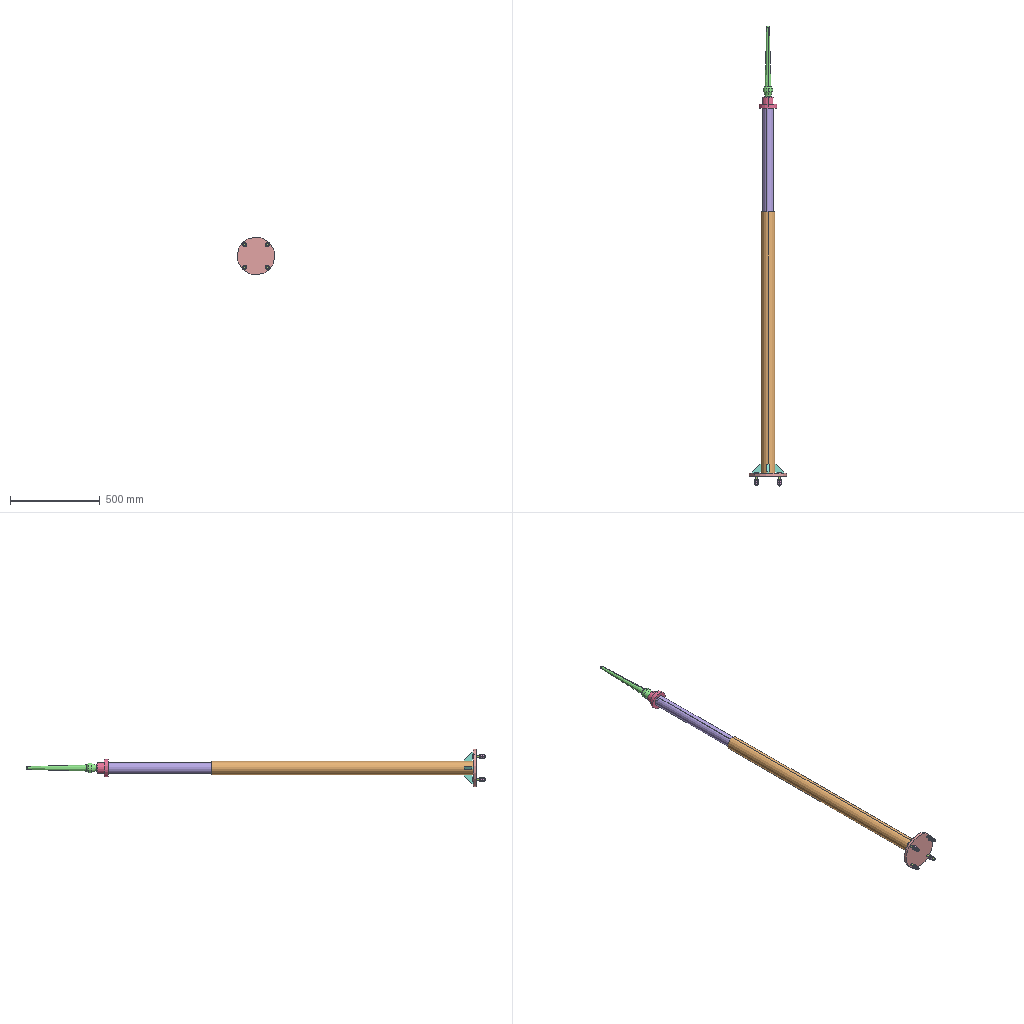Assembly | SolidWorks | 9 different items | 25 placed | box 209 x 2568 x 209 mm
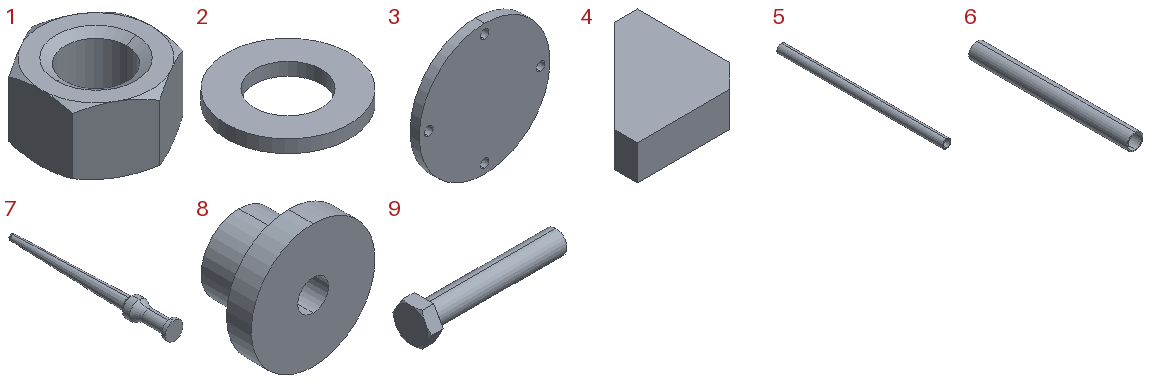Parts list (item | quantity | size | volume | features):
1 | x8 | 18 x 20.785 x 10.8 mm | 2109 mm3 | features ICE 2, RevCut 2, Extrusion 1
2 | x4 | 24 x 24 x 2.5 mm | 799.143 mm3 | features Extrusion 1
3 | x1 | 210 x 15 x 210 mm | 510305 mm3 | features Extrusion 1, HoleWzd 1, RefAxis 1
4 | x4 | 50 x 50 x 15 mm | 24750 mm3 | features Extrusion 1
5 | x1 | 76 x 1460 x 76 mm | 2215388 mm3 | features WeldMemberFeat 1, WeldmentFeature 1
6 | x1 | 60 x 590 x 60 mm | 415193 mm3 | features WeldMemberFeat 1, WeldmentFeature 1
7 | x1 | 54 x 468 x 54 mm | 343926 mm3 | features Revolution 1
8 | x1 | 100 x 60 x 100 mm | 182448 mm3 | features Revolution 1
9 | x4 | 77.5 x 20.785 x 18 mm | 9985 mm3 | features RevCut 3, Extrusion 1, Fillet 1, LPattern 1, Revolution 1
Mates (type | each side: item.copy, entity, surface, feature):
Coincident | 3.1 face plane Boss-Extrude1 | assembly plane
PlanarAngleDim | assembly plane | 3.1 plane
Coincident | 3.1 axis | assembly select_type:11
Concentric | 3.1 face cylinder Boss-Extrude1 | 5.1 face cylinder Gb/t 6728-2002 round tube 76×7(1)
Concentric | 3.1 face cylinder Boss-Extrude1 | 6.1 face cylinder Gb/t 6728-2002 round tube 60 × 4(1)
Concentric | 3.1 face cylinder Boss-Extrude1 | 7.1 face cone Revolve1
Coincident | 3.1 face plane Boss-Extrude1 | 5.1 face plane Gb/t 6728-2002 round tube 76×7(1)
DistanceDim | 5.1 face plane Gb/t 6728-2002 round tube 76×7(1) | 6.1 face plane Gb/t 6728-2002 round tube 60 × 4(1)
Coincident | 6.1 face plane Gb/t 6728-2002 round tube 60 × 4(1) | 7.1 face plane Revolve1
Coincident | 4.1 plane | assembly plane
Coincident | 3.1 face plane Boss-Extrude1 | 4.1 face plane Boss-Extrude1
Tangent | 4.1 face plane Boss-Extrude1 | 5.1 face cylinder Gb/t 6728-2002 round tube 76×7(1)
Concentric | 9.1 face cylinder Boss-Revolve1 | 1.1 face cylinder Boss-Extrude1
Concentric | 9.1 face cylinder Boss-Revolve1 | 1.2 face cylinder Boss-Extrude1
Concentric | 9.1 face cylinder Boss-Revolve1 | 2.1 face cylinder Extrude1
Coincident | 1.1 face plane Boss-Extrude1 | 1.2 face plane Boss-Extrude1 | 2 times
Coincident | 1.1 face plane Boss-Extrude1 | 2.1 face plane Extrude1
Concentric | 3.1 face cylinder Ø14.0 (14) Diameter Hole1 | 9.1 face cylinder Boss-Revolve1
Coincident | 3.1 face plane Boss-Extrude1 | 9.1 face plane Base-Extrude
DistanceDim | 2.1 face plane Extrude1 | 3.1 face plane Boss-Extrude1
Concentric | 7.1 face cylinder Revolve1 | 8.1 face cylinder Revolve1
Coincident | 6.1 edge | 8.1 face plane Revolve1